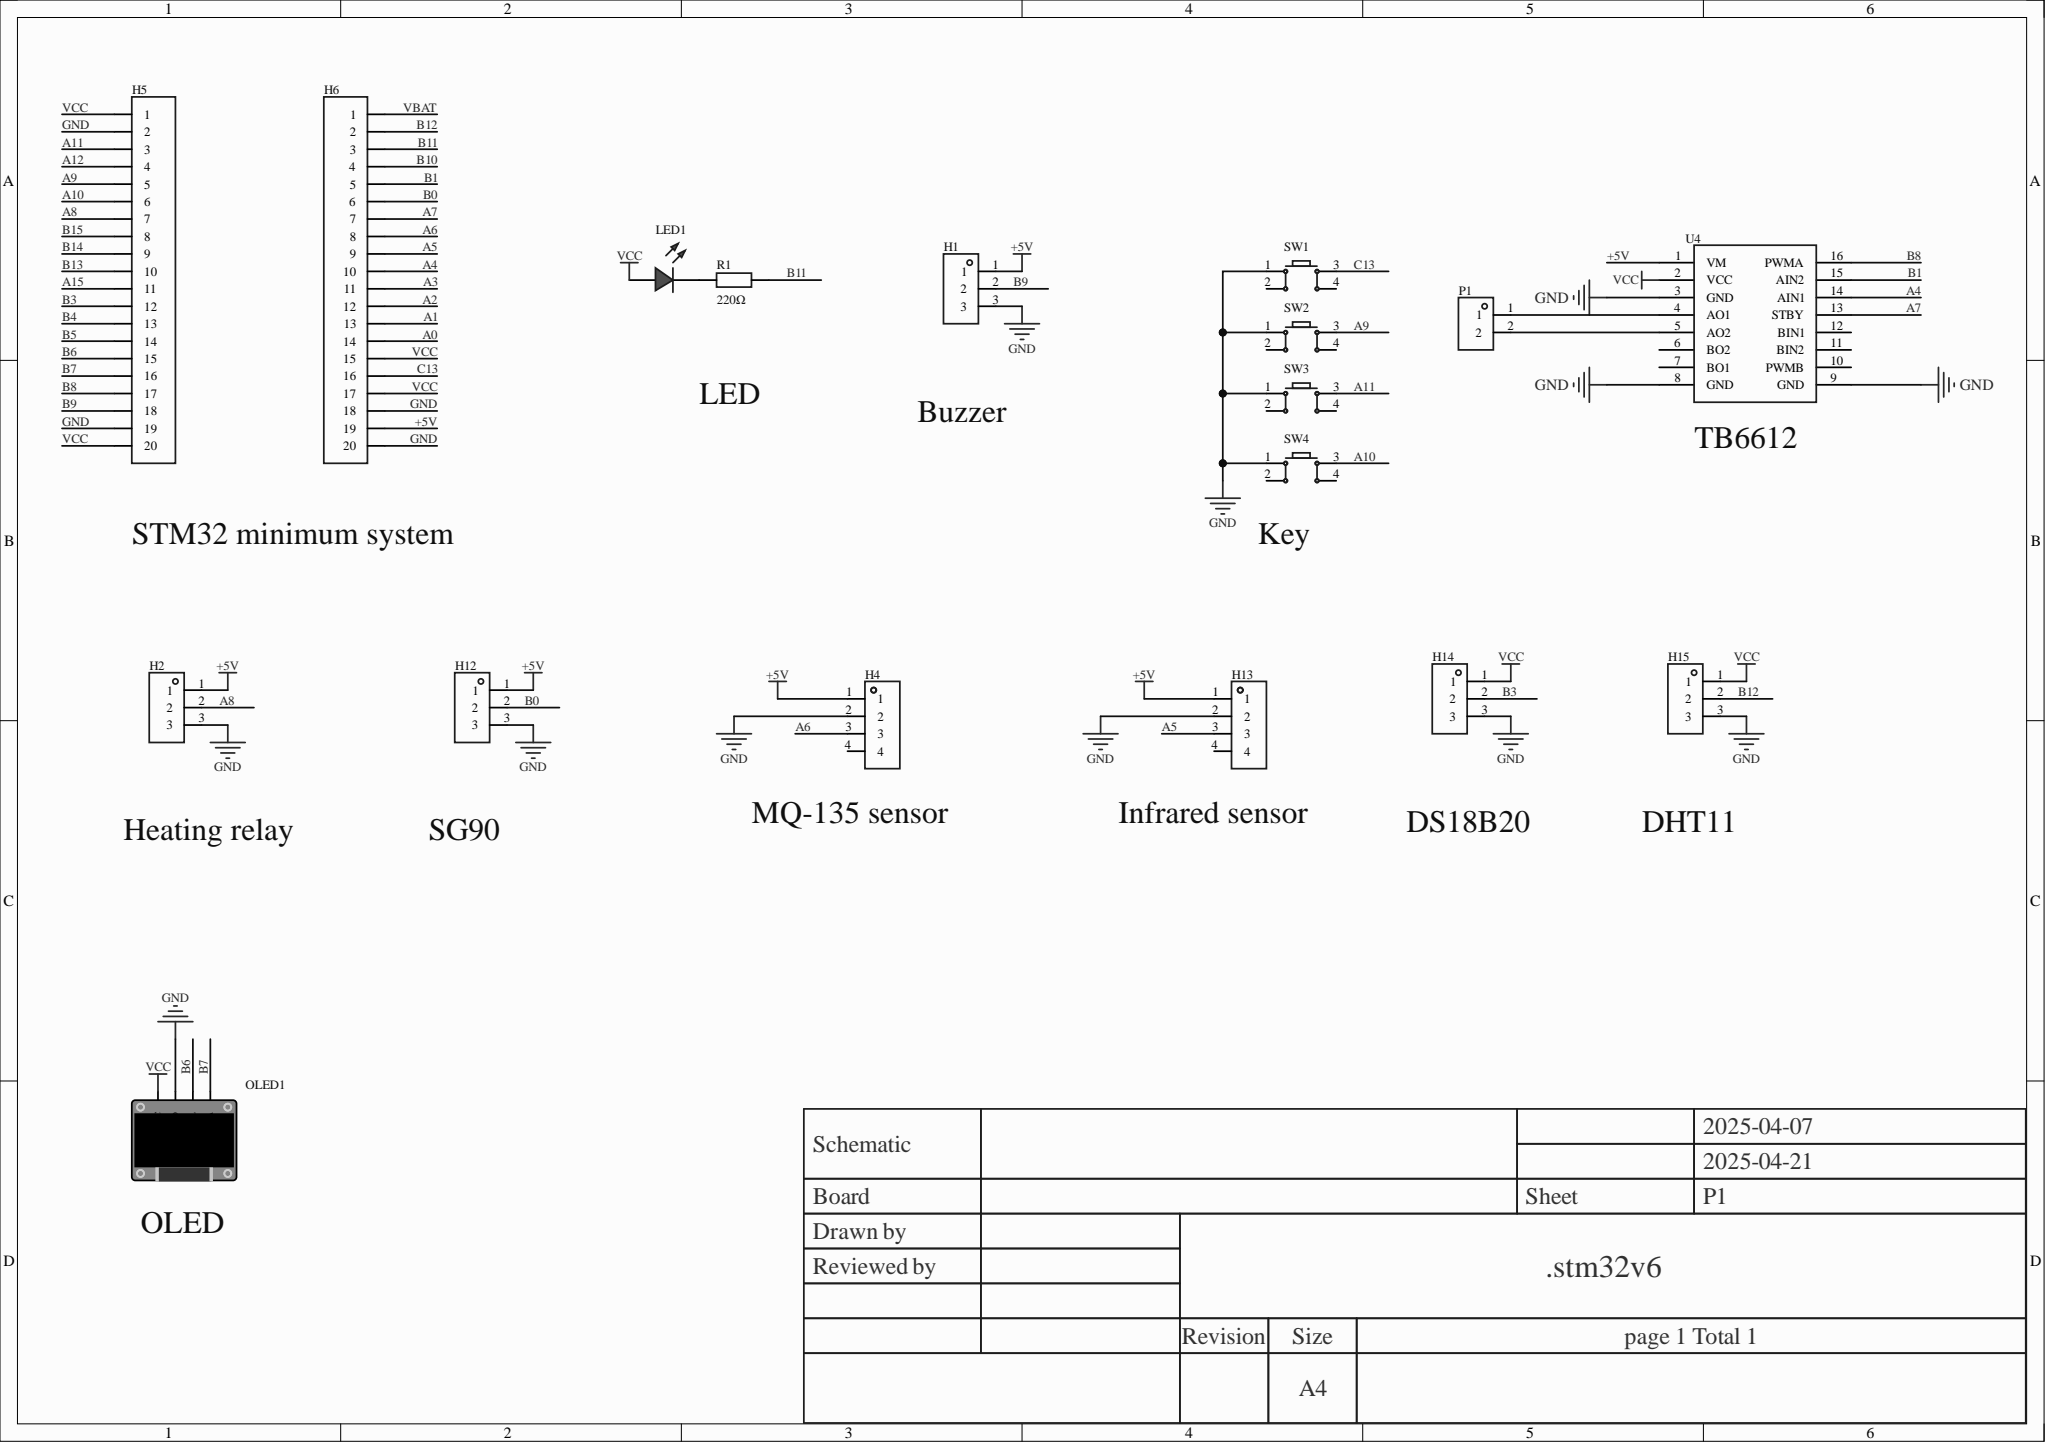Circuit board | Altium Designer | 18 parts | 24 nets
Bill of materials:
Comment,Description,Designator,Footprint,LibRef,Quantity
"","","H1, H2, H12, H14, H15","HDR-TH_3P-P2.54-V-F","HDR-F_2.54_1x3P","5"
"","","H4, H13","HDR-TH_4P-P2.54-V-F","HDR-F_2.54_1x4P","2"
"","","H5, H6","HDR-TH_20P-P2.54-V-F","HDR-F_2.54_1x20P","2"
"","","LED1","LED_TH-3mm","LED_TH-R_3mm","1"
"","","OLED1","0.96OLED_4P","0.96OLED模块_4P","1"
"KF301-2P terminal block","","P1","CONN-TH_XY301V-A-5.0-2P","KF301-2P接线端子","1"
"220Ω","","R1","Res_1/8W","Res_AXIAL-1/8W","1"
"","","SW1, SW2, SW3, SW4","SW-TH_4P-L6.0-W6.0-P4.50-LS6.5","Key_TH_6x6x6","4"
"","","U4","tb6612","tb6612","1"
Netlist (Protel format):
[
H1
HDR-TH_3P-P2.54-V-F




]
[
H2
HDR-TH_3P-P2.54-V-F




]
[
H4
HDR-TH_4P-P2.54-V-F




]
[
H5
HDR-TH_20P-P2.54-V-F




]
[
H6
HDR-TH_20P-P2.54-V-F




]
[
H12
HDR-TH_3P-P2.54-V-F




]
[
H13
HDR-TH_4P-P2.54-V-F




]
[
H14
HDR-TH_3P-P2.54-V-F




]
[
H15
HDR-TH_3P-P2.54-V-F




]
[
LED1
LED_TH-3mm




]
[
OLED1
0.96OLED_4P




]
[
P1
CONN-TH_XY301V-A-5.0-2P
KF301-2P terminal block



]
[
R1
Res_1/8W
220Ω



]
[
SW1
SW-TH_4P-L6.0-W6.0-P4.50-LS6.5




]
[
SW2
SW-TH_4P-L6.0-W6.0-P4.50-LS6.5




]
[
SW3
SW-TH_4P-L6.0-W6.0-P4.50-LS6.5




]
[
SW4
SW-TH_4P-L6.0-W6.0-P4.50-LS6.5




]
[
U4
tb6612




]
(
VCC
H5-1
H5-20
H6-15
H6-17
H14-1
H15-1
LED1-1
OLED1-1
U4-2
)
(
NetP1_2
P1-2
U4-5
)
(
NetP1_1
P1-1
U4-4
)
(
NetLED1_2
LED1-2
R1-1
)
(
GND
H1-3
H2-3
H4-2
H5-2
H5-19
H6-18
H6-20
H12-3
H13-2
H14-3
H15-3
OLED1-2
SW1-1
SW2-1
SW3-1
SW4-1
U4-3
U4-8
U4-9
)
(
C13
H6-16
SW1-3
)
(
B12
H6-2
H15-2
)
(
B11
H6-3
R1-2
)
(
B9
H1-2
H5-18
)
(
B8
H5-17
U4-16
)
(
B7
H5-16
OLED1-4
)
(
B6
H5-15
OLED1-3
)
(
B3
H5-12
H14-2
)
(
B1
H6-5
U4-15
)
(
B0
H6-6
H12-2
)
(
A11
H5-3
SW3-3
)
(
A10
H5-6
SW4-3
)
(
A9
H5-5
SW2-3
)
(
A8
H2-2
H5-7
)
(
A7
H6-7
U4-13
)
(
A6
H4-3
H6-8
)
(
A5
H6-9
H13-3
)
(
A4
H6-10
U4-14
)
(
+5V
H1-1
H2-1
H4-1
H6-19
H12-1
H13-1
U4-1
)